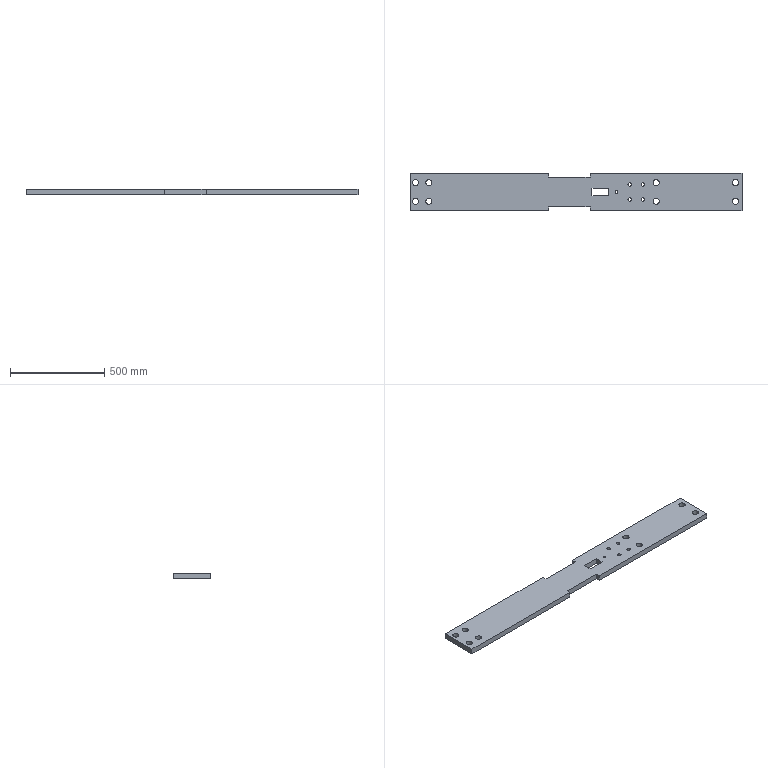Part | NX | features BREP 1, DATUM_CSYS 1, SKETCH 1 | 1 solid | 44 faces | box 1759 x 200 x 30 mm | volume 9929100 mm3 | cylinder 26 | plane 18 | commonest cylinder face diameters 18 x8 32 x8 33 x8 14 x2
STEP:
#1=CARTESIAN_POINT('',(-427.,0.,0.));
#2=VERTEX_POINT('',#1);
#3=CARTESIAN_POINT('',(-413.,0.,0.));
#4=VERTEX_POINT('',#3);
#5=CARTESIAN_POINT('',(-420.,0.,0.));
#6=DIRECTION('',(0.,0.,1.));
#7=DIRECTION('',(1.,0.,0.));
#8=AXIS2_PLACEMENT_3D('',#5,#6,#7);
#9=CIRCLE('',#8,7.);
#10=EDGE_CURVE('',#2,#4,#9,.T.);
#11=ORIENTED_EDGE('',*,*,#10,.F.);
#12=CARTESIAN_POINT('',(-427.,0.,30.));
#13=VERTEX_POINT('',#12);
#14=CARTESIAN_POINT('',(-427.,0.,0.));
#15=DIRECTION('',(0.,0.,1.));
#16=VECTOR('',#15,1000.);
#17=LINE('',#14,#16);
#18=EDGE_CURVE('',#2,#13,#17,.T.);
#19=ORIENTED_EDGE('',*,*,#18,.T.);
#20=CARTESIAN_POINT('',(-413.,0.,30.));
#21=VERTEX_POINT('',#20);
#22=CARTESIAN_POINT('',(-420.,0.,30.));
#23=DIRECTION('',(0.,0.,1.));
#24=DIRECTION('',(1.,0.,0.));
#25=AXIS2_PLACEMENT_3D('',#22,#23,#24);
#26=CIRCLE('',#25,7.);
#27=EDGE_CURVE('',#13,#21,#26,.T.);
#28=ORIENTED_EDGE('',*,*,#27,.T.);
#29=CARTESIAN_POINT('',(-413.,0.,0.));
#30=DIRECTION('',(0.,0.,1.));
#31=VECTOR('',#30,1000.);
#32=LINE('',#29,#31);
#33=EDGE_CURVE('',#4,#21,#32,.T.);
#34=ORIENTED_EDGE('',*,*,#33,.F.);
#35=EDGE_LOOP('',(#11,#19,#28,#34));
#36=FACE_BOUND('',#35,.T.);
#37=CARTESIAN_POINT('',(-420.,0.,0.));
#38=DIRECTION('',(0.,0.,1.));
#39=DIRECTION('',(-1.,0.,0.));
#40=AXIS2_PLACEMENT_3D('',#37,#38,#39);
#41=CYLINDRICAL_SURFACE('',#40,7.);
#42=ADVANCED_FACE('',(#36),#41,.F.);
#43=CARTESIAN_POINT('',(-1500.,50.,30.));
#44=VERTEX_POINT('',#43);
#45=CARTESIAN_POINT('',(-1468.,50.,30.));
#46=VERTEX_POINT('',#45);
#47=CARTESIAN_POINT('',(-1484.,50.,30.));
#48=DIRECTION('',(0.,0.,1.));
#49=DIRECTION('',(1.,0.,0.));
#50=AXIS2_PLACEMENT_3D('',#47,#48,#49);
#51=CIRCLE('',#50,16.);
#52=EDGE_CURVE('',#44,#46,#51,.T.);
#53=ORIENTED_EDGE('',*,*,#52,.T.);
#54=CARTESIAN_POINT('',(-1468.,50.,0.));
#55=VERTEX_POINT('',#54);
#56=CARTESIAN_POINT('',(-1468.,50.,30.));
#57=DIRECTION('',(0.,0.,-1.));
#58=VECTOR('',#57,1000.);
#59=LINE('',#56,#58);
#60=EDGE_CURVE('',#55,#46,#59,.F.);
#61=ORIENTED_EDGE('',*,*,#60,.F.);
#62=CARTESIAN_POINT('',(-1500.,50.,0.));
#63=VERTEX_POINT('',#62);
#64=CARTESIAN_POINT('',(-1484.,50.,0.));
#65=DIRECTION('',(0.,0.,1.));
#66=DIRECTION('',(1.,0.,0.));
#67=AXIS2_PLACEMENT_3D('',#64,#65,#66);
#68=CIRCLE('',#67,16.);
#69=EDGE_CURVE('',#63,#55,#68,.T.);
#70=ORIENTED_EDGE('',*,*,#69,.F.);
#71=CARTESIAN_POINT('',(-1500.,50.,30.));
#72=DIRECTION('',(0.,0.,-1.));
#73=VECTOR('',#72,1000.);
#74=LINE('',#71,#73);
#75=EDGE_CURVE('',#63,#44,#74,.F.);
#76=ORIENTED_EDGE('',*,*,#75,.T.);
#77=EDGE_LOOP('',(#53,#61,#70,#76));
#78=FACE_BOUND('',#77,.T.);
#79=CARTESIAN_POINT('',(-1484.,50.,30.));
#80=DIRECTION('',(0.,0.,-1.));
#81=DIRECTION('',(1.,0.,0.));
#82=AXIS2_PLACEMENT_3D('',#79,#80,#81);
#83=CYLINDRICAL_SURFACE('',#82,16.);
#84=ADVANCED_FACE('',(#78),#83,.F.);
#85=CARTESIAN_POINT('',(-1500.,-50.,30.));
#86=VERTEX_POINT('',#85);
#87=CARTESIAN_POINT('',(-1468.,-50.,30.));
#88=VERTEX_POINT('',#87);
#89=CARTESIAN_POINT('',(-1484.,-50.,30.));
#90=DIRECTION('',(0.,0.,1.));
#91=DIRECTION('',(1.,0.,0.));
#92=AXIS2_PLACEMENT_3D('',#89,#90,#91);
#93=CIRCLE('',#92,16.);
#94=EDGE_CURVE('',#86,#88,#93,.T.);
#95=ORIENTED_EDGE('',*,*,#94,.T.);
#96=CARTESIAN_POINT('',(-1468.,-50.,0.));
#97=VERTEX_POINT('',#96);
#98=CARTESIAN_POINT('',(-1468.,-50.,30.));
#99=DIRECTION('',(0.,0.,-1.));
#100=VECTOR('',#99,1000.);
#101=LINE('',#98,#100);
#102=EDGE_CURVE('',#97,#88,#101,.F.);
#103=ORIENTED_EDGE('',*,*,#102,.F.);
#104=CARTESIAN_POINT('',(-1500.,-50.,0.));
#105=VERTEX_POINT('',#104);
#106=CARTESIAN_POINT('',(-1484.,-50.,0.));
#107=DIRECTION('',(0.,0.,1.));
#108=DIRECTION('',(1.,0.,0.));
#109=AXIS2_PLACEMENT_3D('',#106,#107,#108);
#110=CIRCLE('',#109,16.);
#111=EDGE_CURVE('',#105,#97,#110,.T.);
#112=ORIENTED_EDGE('',*,*,#111,.F.);
#113=CARTESIAN_POINT('',(-1500.,-50.,30.));
#114=DIRECTION('',(0.,0.,-1.));
#115=VECTOR('',#114,1000.);
#116=LINE('',#113,#115);
#117=EDGE_CURVE('',#105,#86,#116,.F.);
#118=ORIENTED_EDGE('',*,*,#117,.T.);
#119=EDGE_LOOP('',(#95,#103,#112,#118));
#120=FACE_BOUND('',#119,.T.);
#121=CARTESIAN_POINT('',(-1484.,-50.,30.));
#122=DIRECTION('',(0.,0.,-1.));
#123=DIRECTION('',(1.,0.,0.));
#124=AXIS2_PLACEMENT_3D('',#121,#122,#123);
#125=CYLINDRICAL_SURFACE('',#124,16.);
#126=ADVANCED_FACE('',(#120),#125,.F.);
#127=CARTESIAN_POINT('',(-1430.,-50.,30.));
#128=VERTEX_POINT('',#127);
#129=CARTESIAN_POINT('',(-1398.,-50.,30.));
#130=VERTEX_POINT('',#129);
#131=CARTESIAN_POINT('',(-1414.,-50.,30.));
#132=DIRECTION('',(0.,0.,1.));
#133=DIRECTION('',(1.,0.,0.));
#134=AXIS2_PLACEMENT_3D('',#131,#132,#133);
#135=CIRCLE('',#134,16.);
#136=EDGE_CURVE('',#128,#130,#135,.T.);
#137=ORIENTED_EDGE('',*,*,#136,.T.);
#138=CARTESIAN_POINT('',(-1398.,-50.,0.));
#139=VERTEX_POINT('',#138);
#140=CARTESIAN_POINT('',(-1398.,-50.,30.));
#141=DIRECTION('',(0.,0.,-1.));
#142=VECTOR('',#141,1000.);
#143=LINE('',#140,#142);
#144=EDGE_CURVE('',#139,#130,#143,.F.);
#145=ORIENTED_EDGE('',*,*,#144,.F.);
#146=CARTESIAN_POINT('',(-1430.,-50.,0.));
#147=VERTEX_POINT('',#146);
#148=CARTESIAN_POINT('',(-1414.,-50.,0.));
#149=DIRECTION('',(0.,0.,1.));
#150=DIRECTION('',(1.,0.,0.));
#151=AXIS2_PLACEMENT_3D('',#148,#149,#150);
#152=CIRCLE('',#151,16.);
#153=EDGE_CURVE('',#147,#139,#152,.T.);
#154=ORIENTED_EDGE('',*,*,#153,.F.);
#155=CARTESIAN_POINT('',(-1430.,-50.,30.));
#156=DIRECTION('',(0.,0.,-1.));
#157=VECTOR('',#156,1000.);
#158=LINE('',#155,#157);
#159=EDGE_CURVE('',#147,#128,#158,.F.);
#160=ORIENTED_EDGE('',*,*,#159,.T.);
#161=EDGE_LOOP('',(#137,#145,#154,#160));
#162=FACE_BOUND('',#161,.T.);
#163=CARTESIAN_POINT('',(-1414.,-50.,30.));
#164=DIRECTION('',(0.,0.,-1.));
#165=DIRECTION('',(1.,0.,0.));
#166=AXIS2_PLACEMENT_3D('',#163,#164,#165);
#167=CYLINDRICAL_SURFACE('',#166,16.);
#168=ADVANCED_FACE('',(#162),#167,.F.);
#169=CARTESIAN_POINT('',(-1430.,50.,30.));
#170=VERTEX_POINT('',#169);
#171=CARTESIAN_POINT('',(-1398.,50.,30.));
#172=VERTEX_POINT('',#171);
#173=CARTESIAN_POINT('',(-1414.,50.,30.));
#174=DIRECTION('',(0.,0.,1.));
#175=DIRECTION('',(1.,0.,0.));
#176=AXIS2_PLACEMENT_3D('',#173,#174,#175);
#177=CIRCLE('',#176,16.);
#178=EDGE_CURVE('',#170,#172,#177,.T.);
#179=ORIENTED_EDGE('',*,*,#178,.T.);
#180=CARTESIAN_POINT('',(-1398.,50.,0.));
#181=VERTEX_POINT('',#180);
#182=CARTESIAN_POINT('',(-1398.,50.,30.));
#183=DIRECTION('',(0.,0.,-1.));
#184=VECTOR('',#183,1000.);
#185=LINE('',#182,#184);
#186=EDGE_CURVE('',#181,#172,#185,.F.);
#187=ORIENTED_EDGE('',*,*,#186,.F.);
#188=CARTESIAN_POINT('',(-1430.,50.,0.));
#189=VERTEX_POINT('',#188);
#190=CARTESIAN_POINT('',(-1414.,50.,0.));
#191=DIRECTION('',(0.,0.,1.));
#192=DIRECTION('',(1.,0.,0.));
#193=AXIS2_PLACEMENT_3D('',#190,#191,#192);
#194=CIRCLE('',#193,16.);
#195=EDGE_CURVE('',#189,#181,#194,.T.);
#196=ORIENTED_EDGE('',*,*,#195,.F.);
#197=CARTESIAN_POINT('',(-1430.,50.,30.));
#198=DIRECTION('',(0.,0.,-1.));
#199=VECTOR('',#198,1000.);
#200=LINE('',#197,#199);
#201=EDGE_CURVE('',#189,#170,#200,.F.);
#202=ORIENTED_EDGE('',*,*,#201,.T.);
#203=EDGE_LOOP('',(#179,#187,#196,#202));
#204=FACE_BOUND('',#203,.T.);
#205=CARTESIAN_POINT('',(-1414.,50.,30.));
#206=DIRECTION('',(0.,0.,-1.));
#207=DIRECTION('',(1.,0.,0.));
#208=AXIS2_PLACEMENT_3D('',#205,#206,#207);
#209=CYLINDRICAL_SURFACE('',#208,16.);
#210=ADVANCED_FACE('',(#204),#209,.F.);
#211=CARTESIAN_POINT('',(-359.,-40.,30.));
#212=VERTEX_POINT('',#211);
#213=CARTESIAN_POINT('',(-341.,-40.,30.));
#214=VERTEX_POINT('',#213);
#215=CARTESIAN_POINT('',(-350.,-40.,30.));
#216=DIRECTION('',(0.,0.,1.));
#217=DIRECTION('',(1.,0.,0.));
#218=AXIS2_PLACEMENT_3D('',#215,#216,#217);
#219=CIRCLE('',#218,9.);
#220=EDGE_CURVE('',#212,#214,#219,.T.);
#221=ORIENTED_EDGE('',*,*,#220,.T.);
#222=CARTESIAN_POINT('',(-341.,-40.,0.));
#223=VERTEX_POINT('',#222);
#224=CARTESIAN_POINT('',(-341.,-40.,30.));
#225=DIRECTION('',(0.,0.,-1.));
#226=VECTOR('',#225,1000.);
#227=LINE('',#224,#226);
#228=EDGE_CURVE('',#223,#214,#227,.F.);
#229=ORIENTED_EDGE('',*,*,#228,.F.);
#230=CARTESIAN_POINT('',(-359.,-40.,0.));
#231=VERTEX_POINT('',#230);
#232=CARTESIAN_POINT('',(-350.,-40.,0.));
#233=DIRECTION('',(0.,0.,1.));
#234=DIRECTION('',(1.,0.,0.));
#235=AXIS2_PLACEMENT_3D('',#232,#233,#234);
#236=CIRCLE('',#235,9.);
#237=EDGE_CURVE('',#231,#223,#236,.T.);
#238=ORIENTED_EDGE('',*,*,#237,.F.);
#239=CARTESIAN_POINT('',(-359.,-40.,30.));
#240=DIRECTION('',(0.,0.,-1.));
#241=VECTOR('',#240,1000.);
#242=LINE('',#239,#241);
#243=EDGE_CURVE('',#231,#212,#242,.F.);
#244=ORIENTED_EDGE('',*,*,#243,.T.);
#245=EDGE_LOOP('',(#221,#229,#238,#244));
#246=FACE_BOUND('',#245,.T.);
#247=CARTESIAN_POINT('',(-350.,-40.,30.));
#248=DIRECTION('',(0.,0.,-1.));
#249=DIRECTION('',(1.,0.,0.));
#250=AXIS2_PLACEMENT_3D('',#247,#248,#249);
#251=CYLINDRICAL_SURFACE('',#250,9.);
#252=ADVANCED_FACE('',(#246),#251,.F.);
#253=CARTESIAN_POINT('',(-289.,-40.,30.));
#254=VERTEX_POINT('',#253);
#255=CARTESIAN_POINT('',(-271.,-40.,30.));
#256=VERTEX_POINT('',#255);
#257=CARTESIAN_POINT('',(-280.,-40.,30.));
#258=DIRECTION('',(0.,0.,1.));
#259=DIRECTION('',(1.,0.,0.));
#260=AXIS2_PLACEMENT_3D('',#257,#258,#259);
#261=CIRCLE('',#260,9.);
#262=EDGE_CURVE('',#254,#256,#261,.T.);
#263=ORIENTED_EDGE('',*,*,#262,.T.);
#264=CARTESIAN_POINT('',(-271.,-40.,0.));
#265=VERTEX_POINT('',#264);
#266=CARTESIAN_POINT('',(-271.,-40.,30.));
#267=DIRECTION('',(0.,0.,-1.));
#268=VECTOR('',#267,1000.);
#269=LINE('',#266,#268);
#270=EDGE_CURVE('',#265,#256,#269,.F.);
#271=ORIENTED_EDGE('',*,*,#270,.F.);
#272=CARTESIAN_POINT('',(-289.,-40.,0.));
#273=VERTEX_POINT('',#272);
#274=CARTESIAN_POINT('',(-280.,-40.,0.));
#275=DIRECTION('',(0.,0.,1.));
#276=DIRECTION('',(1.,0.,0.));
#277=AXIS2_PLACEMENT_3D('',#274,#275,#276);
#278=CIRCLE('',#277,9.);
#279=EDGE_CURVE('',#273,#265,#278,.T.);
#280=ORIENTED_EDGE('',*,*,#279,.F.);
#281=CARTESIAN_POINT('',(-289.,-40.,30.));
#282=DIRECTION('',(0.,0.,-1.));
#283=VECTOR('',#282,1000.);
#284=LINE('',#281,#283);
#285=EDGE_CURVE('',#273,#254,#284,.F.);
#286=ORIENTED_EDGE('',*,*,#285,.T.);
#287=EDGE_LOOP('',(#263,#271,#280,#286));
#288=FACE_BOUND('',#287,.T.);
#289=CARTESIAN_POINT('',(-280.,-40.,30.));
#290=DIRECTION('',(0.,0.,-1.));
#291=DIRECTION('',(1.,0.,0.));
#292=AXIS2_PLACEMENT_3D('',#289,#290,#291);
#293=CYLINDRICAL_SURFACE('',#292,9.);
#294=ADVANCED_FACE('',(#288),#293,.F.);
#295=CARTESIAN_POINT('',(-289.,40.,30.));
#296=VERTEX_POINT('',#295);
#297=CARTESIAN_POINT('',(-271.,40.,30.));
#298=VERTEX_POINT('',#297);
#299=CARTESIAN_POINT('',(-280.,40.,30.));
#300=DIRECTION('',(0.,0.,1.));
#301=DIRECTION('',(1.,0.,0.));
#302=AXIS2_PLACEMENT_3D('',#299,#300,#301);
#303=CIRCLE('',#302,9.);
#304=EDGE_CURVE('',#296,#298,#303,.T.);
#305=ORIENTED_EDGE('',*,*,#304,.T.);
#306=CARTESIAN_POINT('',(-271.,40.,0.));
#307=VERTEX_POINT('',#306);
#308=CARTESIAN_POINT('',(-271.,40.,30.));
#309=DIRECTION('',(0.,0.,-1.));
#310=VECTOR('',#309,1000.);
#311=LINE('',#308,#310);
#312=EDGE_CURVE('',#307,#298,#311,.F.);
#313=ORIENTED_EDGE('',*,*,#312,.F.);
#314=CARTESIAN_POINT('',(-289.,40.,0.));
#315=VERTEX_POINT('',#314);
#316=CARTESIAN_POINT('',(-280.,40.,0.));
#317=DIRECTION('',(0.,0.,1.));
#318=DIRECTION('',(1.,0.,0.));
#319=AXIS2_PLACEMENT_3D('',#316,#317,#318);
#320=CIRCLE('',#319,9.);
#321=EDGE_CURVE('',#315,#307,#320,.T.);
#322=ORIENTED_EDGE('',*,*,#321,.F.);
#323=CARTESIAN_POINT('',(-289.,40.,30.));
#324=DIRECTION('',(0.,0.,-1.));
#325=VECTOR('',#324,1000.);
#326=LINE('',#323,#325);
#327=EDGE_CURVE('',#315,#296,#326,.F.);
#328=ORIENTED_EDGE('',*,*,#327,.T.);
#329=EDGE_LOOP('',(#305,#313,#322,#328));
#330=FACE_BOUND('',#329,.T.);
#331=CARTESIAN_POINT('',(-280.,40.,30.));
#332=DIRECTION('',(0.,0.,-1.));
#333=DIRECTION('',(1.,0.,0.));
#334=AXIS2_PLACEMENT_3D('',#331,#332,#333);
#335=CYLINDRICAL_SURFACE('',#334,9.);
#336=ADVANCED_FACE('',(#330),#335,.F.);
#337=CARTESIAN_POINT('',(-359.,40.,30.));
#338=VERTEX_POINT('',#337);
#339=CARTESIAN_POINT('',(-341.,40.,30.));
#340=VERTEX_POINT('',#339);
#341=CARTESIAN_POINT('',(-350.,40.,30.));
#342=DIRECTION('',(0.,0.,1.));
#343=DIRECTION('',(1.,0.,0.));
#344=AXIS2_PLACEMENT_3D('',#341,#342,#343);
#345=CIRCLE('',#344,9.);
#346=EDGE_CURVE('',#338,#340,#345,.T.);
#347=ORIENTED_EDGE('',*,*,#346,.T.);
#348=CARTESIAN_POINT('',(-341.,40.,0.));
#349=VERTEX_POINT('',#348);
#350=CARTESIAN_POINT('',(-341.,40.,30.));
#351=DIRECTION('',(0.,0.,-1.));
#352=VECTOR('',#351,1000.);
#353=LINE('',#350,#352);
#354=EDGE_CURVE('',#349,#340,#353,.F.);
#355=ORIENTED_EDGE('',*,*,#354,.F.);
#356=CARTESIAN_POINT('',(-359.,40.,0.));
#357=VERTEX_POINT('',#356);
#358=CARTESIAN_POINT('',(-350.,40.,0.));
#359=DIRECTION('',(0.,0.,1.));
#360=DIRECTION('',(1.,0.,0.));
#361=AXIS2_PLACEMENT_3D('',#358,#359,#360);
#362=CIRCLE('',#361,9.);
#363=EDGE_CURVE('',#357,#349,#362,.T.);
#364=ORIENTED_EDGE('',*,*,#363,.F.);
#365=CARTESIAN_POINT('',(-359.,40.,30.));
#366=DIRECTION('',(0.,0.,-1.));
#367=VECTOR('',#366,1000.);
#368=LINE('',#365,#367);
#369=EDGE_CURVE('',#357,#338,#368,.F.);
#370=ORIENTED_EDGE('',*,*,#369,.T.);
#371=EDGE_LOOP('',(#347,#355,#364,#370));
#372=FACE_BOUND('',#371,.T.);
#373=CARTESIAN_POINT('',(-350.,40.,30.));
#374=DIRECTION('',(0.,0.,-1.));
#375=DIRECTION('',(1.,0.,0.));
#376=AXIS2_PLACEMENT_3D('',#373,#374,#375);
#377=CYLINDRICAL_SURFACE('',#376,9.);
#378=ADVANCED_FACE('',(#372),#377,.F.);
#379=CARTESIAN_POINT('',(-226.5,50.,30.));
#380=VERTEX_POINT('',#379);
#381=CARTESIAN_POINT('',(-193.5,50.,30.));
#382=VERTEX_POINT('',#381);
#383=CARTESIAN_POINT('',(-210.,50.,30.));
#384=DIRECTION('',(0.,0.,1.));
#385=DIRECTION('',(1.,0.,0.));
#386=AXIS2_PLACEMENT_3D('',#383,#384,#385);
#387=CIRCLE('',#386,16.5);
#388=EDGE_CURVE('',#380,#382,#387,.T.);
#389=ORIENTED_EDGE('',*,*,#388,.T.);
#390=CARTESIAN_POINT('',(-193.5,50.,0.));
#391=VERTEX_POINT('',#390);
#392=CARTESIAN_POINT('',(-193.5,50.,30.));
#393=DIRECTION('',(0.,0.,-1.));
#394=VECTOR('',#393,1000.);
#395=LINE('',#392,#394);
#396=EDGE_CURVE('',#391,#382,#395,.F.);
#397=ORIENTED_EDGE('',*,*,#396,.F.);
#398=CARTESIAN_POINT('',(-226.5,50.,0.));
#399=VERTEX_POINT('',#398);
#400=CARTESIAN_POINT('',(-210.,50.,0.));
#401=DIRECTION('',(0.,0.,1.));
#402=DIRECTION('',(1.,0.,0.));
#403=AXIS2_PLACEMENT_3D('',#400,#401,#402);
#404=CIRCLE('',#403,16.5);
#405=EDGE_CURVE('',#399,#391,#404,.T.);
#406=ORIENTED_EDGE('',*,*,#405,.F.);
#407=CARTESIAN_POINT('',(-226.5,50.,30.));
#408=DIRECTION('',(0.,0.,-1.));
#409=VECTOR('',#408,1000.);
#410=LINE('',#407,#409);
#411=EDGE_CURVE('',#399,#380,#410,.F.);
#412=ORIENTED_EDGE('',*,*,#411,.T.);
#413=EDGE_LOOP('',(#389,#397,#406,#412));
#414=FACE_BOUND('',#413,.T.);
#415=CARTESIAN_POINT('',(-210.,50.,30.));
#416=DIRECTION('',(0.,0.,-1.));
#417=DIRECTION('',(1.,0.,0.));
#418=AXIS2_PLACEMENT_3D('',#415,#416,#417);
#419=CYLINDRICAL_SURFACE('',#418,16.5);
#420=ADVANCED_FACE('',(#414),#419,.F.);
#421=CARTESIAN_POINT('',(-226.5,-50.,30.));
#422=VERTEX_POINT('',#421);
#423=CARTESIAN_POINT('',(-193.5,-50.,30.));
#424=VERTEX_POINT('',#423);
#425=CARTESIAN_POINT('',(-210.,-50.,30.));
#426=DIRECTION('',(0.,0.,1.));
#427=DIRECTION('',(1.,0.,0.));
#428=AXIS2_PLACEMENT_3D('',#425,#426,#427);
#429=CIRCLE('',#428,16.5);
#430=EDGE_CURVE('',#422,#424,#429,.T.);
#431=ORIENTED_EDGE('',*,*,#430,.T.);
#432=CARTESIAN_POINT('',(-193.5,-50.,0.));
#433=VERTEX_POINT('',#432);
#434=CARTESIAN_POINT('',(-193.5,-50.,30.));
#435=DIRECTION('',(0.,0.,-1.));
#436=VECTOR('',#435,1000.);
#437=LINE('',#434,#436);
#438=EDGE_CURVE('',#433,#424,#437,.F.);
#439=ORIENTED_EDGE('',*,*,#438,.F.);
#440=CARTESIAN_POINT('',(-226.5,-50.,0.));
#441=VERTEX_POINT('',#440);
#442=CARTESIAN_POINT('',(-210.,-50.,0.));
#443=DIRECTION('',(0.,0.,1.));
#444=DIRECTION('',(1.,0.,0.));
#445=AXIS2_PLACEMENT_3D('',#442,#443,#444);
#446=CIRCLE('',#445,16.5);
#447=EDGE_CURVE('',#441,#433,#446,.T.);
#448=ORIENTED_EDGE('',*,*,#447,.F.);
#449=CARTESIAN_POINT('',(-226.5,-50.,30.));
#450=DIRECTION('',(0.,0.,-1.));
#451=VECTOR('',#450,1000.);
#452=LINE('',#449,#451);
#453=EDGE_CURVE('',#441,#422,#452,.F.);
#454=ORIENTED_EDGE('',*,*,#453,.T.);
#455=EDGE_LOOP('',(#431,#439,#448,#454));
#456=FACE_BOUND('',#455,.T.);
#457=CARTESIAN_POINT('',(-210.,-50.,30.));
#458=DIRECTION('',(0.,0.,-1.));
#459=DIRECTION('',(1.,0.,0.));
#460=AXIS2_PLACEMENT_3D('',#457,#458,#459);
#461=CYLINDRICAL_SURFACE('',#460,16.5);
#462=ADVANCED_FACE('',(#456),#461,.F.);
#463=CARTESIAN_POINT('',(193.5,-50.,30.));
#464=VERTEX_POINT('',#463);
#465=CARTESIAN_POINT('',(226.5,-50.,30.));
#466=VERTEX_POINT('',#465);
#467=CARTESIAN_POINT('',(210.,-50.,30.));
#468=DIRECTION('',(0.,0.,1.));
#469=DIRECTION('',(1.,0.,0.));
#470=AXIS2_PLACEMENT_3D('',#467,#468,#469);
#471=CIRCLE('',#470,16.5);
#472=EDGE_CURVE('',#464,#466,#471,.T.);
#473=ORIENTED_EDGE('',*,*,#472,.T.);
#474=CARTESIAN_POINT('',(226.5,-50.,0.));
#475=VERTEX_POINT('',#474);
#476=CARTESIAN_POINT('',(226.5,-50.,30.));
#477=DIRECTION('',(0.,0.,-1.));
#478=VECTOR('',#477,1000.);
#479=LINE('',#476,#478);
#480=EDGE_CURVE('',#475,#466,#479,.F.);
#481=ORIENTED_EDGE('',*,*,#480,.F.);
#482=CARTESIAN_POINT('',(193.5,-50.,0.));
#483=VERTEX_POINT('',#482);
#484=CARTESIAN_POINT('',(210.,-50.,0.));
#485=DIRECTION('',(0.,0.,1.));
#486=DIRECTION('',(1.,0.,0.));
#487=AXIS2_PLACEMENT_3D('',#484,#485,#486);
#488=CIRCLE('',#487,16.5);
#489=EDGE_CURVE('',#483,#475,#488,.T.);
#490=ORIENTED_EDGE('',*,*,#489,.F.);
#491=CARTESIAN_POINT('',(193.5,-50.,30.));
#492=DIRECTION('',(0.,0.,-1.));
#493=VECTOR('',#492,1000.);
#494=LINE('',#491,#493);
#495=EDGE_CURVE('',#483,#464,#494,.F.);
#496=ORIENTED_EDGE('',*,*,#495,.T.);
#497=EDGE_LOOP('',(#473,#481,#490,#496));
#498=FACE_BOUND('',#497,.T.);
#499=CARTESIAN_POINT('',(210.,-50.,30.));
#500=DIRECTION('',(0.,0.,-1.));
#501=DIRECTION('',(1.,0.,0.));
#502=AXIS2_PLACEMENT_3D('',#499,#500,#501);
#503=CYLINDRICAL_SURFACE('',#502,16.5);
#504=ADVANCED_FACE('',(#498),#503,.F.);
#505=CARTESIAN_POINT('',(193.5,50.,30.));
#506=VERTEX_POINT('',#505);
#507=CARTESIAN_POINT('',(226.5,50.,30.));
#508=VERTEX_POINT('',#507);
#509=CARTESIAN_POINT('',(210.,50.,30.));
#510=DIRECTION('',(0.,0.,1.));
#511=DIRECTION('',(1.,0.,0.));
#512=AXIS2_PLACEMENT_3D('',#509,#510,#511);
#513=CIRCLE('',#512,16.5);
#514=EDGE_CURVE('',#506,#508,#513,.T.);
#515=ORIENTED_EDGE('',*,*,#514,.T.);
#516=CARTESIAN_POINT('',(226.5,50.,0.));
#517=VERTEX_POINT('',#516);
#518=CARTESIAN_POINT('',(226.5,50.,30.));
#519=DIRECTION('',(0.,0.,-1.));
#520=VECTOR('',#519,1000.);
#521=LINE('',#518,#520);
#522=EDGE_CURVE('',#517,#508,#521,.F.);
#523=ORIENTED_EDGE('',*,*,#522,.F.);
#524=CARTESIAN_POINT('',(193.5,50.,0.));
#525=VERTEX_POINT('',#524);
#526=CARTESIAN_POINT('',(210.,50.,0.));
#527=DIRECTION('',(0.,0.,1.));
#528=DIRECTION('',(1.,0.,0.));
#529=AXIS2_PLACEMENT_3D('',#526,#527,#528);
#530=CIRCLE('',#529,16.5);
#531=EDGE_CURVE('',#525,#517,#530,.T.);
#532=ORIENTED_EDGE('',*,*,#531,.F.);
#533=CARTESIAN_POINT('',(193.5,50.,30.));
#534=DIRECTION('',(0.,0.,-1.));
#535=VECTOR('',#534,1000.);
#536=LINE('',#533,#535);
#537=EDGE_CURVE('',#525,#506,#536,.F.);
#538=ORIENTED_EDGE('',*,*,#537,.T.);
#539=EDGE_LOOP('',(#515,#523,#532,#538));
#540=FACE_BOUND('',#539,.T.);
#541=CARTESIAN_POINT('',(210.,50.,30.));
#542=DIRECTION('',(0.,0.,-1.));
#543=DIRECTION('',(1.,0.,0.));
#544=AXIS2_PLACEMENT_3D('',#541,#542,#543);
#545=CYLINDRICAL_SURFACE('',#544,16.5);
#546=ADVANCED_FACE('',(#540),#545,.F.);
#547=CARTESIAN_POINT('',(-420.,0.,30.));
#548=DIRECTION('',(0.,0.,1.));
#549=DIRECTION('',(1.,0.,0.));
#550=AXIS2_PLACEMENT_3D('',#547,#548,#549);
#551=CIRCLE('',#550,7.);
#552=EDGE_CURVE('',#21,#13,#551,.T.);
#553=ORIENTED_EDGE('',*,*,#552,.F.);
#554=ORIENTED_EDGE('',*,*,#27,.F.);
#555=EDGE_LOOP('',(#553,#554));
#556=FACE_BOUND('',#555,.T.);
#557=CARTESIAN_POINT('',(-550.,-21.,30.));
#558=VERTEX_POINT('',#557);
#559=CARTESIAN_POINT('',(-460.,-21.,30.));
#560=VERTEX_POINT('',#559);
#561=CARTESIAN_POINT('',(-550.,-21.,30.));
#562=DIRECTION('',(1.,0.,0.));
#563=VECTOR('',#562,1000.);
#564=LINE('',#561,#563);
#565=EDGE_CURVE('',#558,#560,#564,.T.);
#566=ORIENTED_EDGE('',*,*,#565,.F.);
#567=CARTESIAN_POINT('',(-550.,21.,30.));
#568=VERTEX_POINT('',#567);
#569=CARTESIAN_POINT('',(-550.,-21.,30.));
#570=DIRECTION('',(0.,-1.,0.));
#571=VECTOR('',#570,1000.);
#572=LINE('',#569,#571);
#573=EDGE_CURVE('',#568,#558,#572,.T.);
#574=ORIENTED_EDGE('',*,*,#573,.F.);
#575=CARTESIAN_POINT('',(-460.,21.,30.));
#576=VERTEX_POINT('',#575);
#577=CARTESIAN_POINT('',(-550.,21.,30.));
#578=DIRECTION('',(-1.,0.,0.));
#579=VECTOR('',#578,1000.);
#580=LINE('',#577,#579);
#581=EDGE_CURVE('',#576,#568,#580,.T.);
#582=ORIENTED_EDGE('',*,*,#581,.F.);
#583=CARTESIAN_POINT('',(-460.,-21.,30.));
#584=DIRECTION('',(0.,1.,0.));
#585=VECTOR('',#584,1000.);
#586=LINE('',#583,#585);
#587=EDGE_CURVE('',#560,#576,#586,.T.);
#588=ORIENTED_EDGE('',*,*,#587,.F.);
#589=EDGE_LOOP('',(#566,#574,#582,#588));
#590=FACE_BOUND('',#589,.T.);
#591=ORIENTED_EDGE('',*,*,#94,.F.);
#592=CARTESIAN_POINT('',(-1484.,-50.,30.));
#593=DIRECTION('',(0.,0.,1.));
#594=DIRECTION('',(1.,0.,0.));
#595=AXIS2_PLACEMENT_3D('',#592,#593,#594);
#596=CIRCLE('',#595,16.);
#597=EDGE_CURVE('',#88,#86,#596,.T.);
#598=ORIENTED_EDGE('',*,*,#597,.F.);
#599=EDGE_LOOP('',(#591,#598));
#600=FACE_BOUND('',#599,.T.);
#601=ORIENTED_EDGE('',*,*,#178,.F.);
#602=CARTESIAN_POINT('',(-1414.,50.,30.));
#603=DIRECTION('',(0.,0.,1.));
#604=DIRECTION('',(1.,0.,0.));
#605=AXIS2_PLACEMENT_3D('',#602,#603,#604);
#606=CIRCLE('',#605,16.);
#607=EDGE_CURVE('',#172,#170,#606,.T.);
#608=ORIENTED_EDGE('',*,*,#607,.F.);
#609=EDGE_LOOP('',(#601,#608));
#610=FACE_BOUND('',#609,.T.);
#611=ORIENTED_EDGE('',*,*,#262,.F.);
#612=CARTESIAN_POINT('',(-280.,-40.,30.));
#613=DIRECTION('',(0.,0.,1.));
#614=DIRECTION('',(1.,0.,0.));
#615=AXIS2_PLACEMENT_3D('',#612,#613,#614);
#616=CIRCLE('',#615,9.);
#617=EDGE_CURVE('',#256,#254,#616,.T.);
#618=ORIENTED_EDGE('',*,*,#617,.F.);
#619=EDGE_LOOP('',(#611,#618));
#620=FACE_BOUND('',#619,.T.);
#621=ORIENTED_EDGE('',*,*,#346,.F.);
#622=CARTESIAN_POINT('',(-350.,40.,30.));
#623=DIRECTION('',(0.,0.,1.));
#624=DIRECTION('',(1.,0.,0.));
#625=AXIS2_PLACEMENT_3D('',#622,#623,#624);
#626=CIRCLE('',#625,9.);
#627=EDGE_CURVE('',#340,#338,#626,.T.);
#628=ORIENTED_EDGE('',*,*,#627,.F.);
#629=EDGE_LOOP('',(#621,#628));
#630=FACE_BOUND('',#629,.T.);
#631=ORIENTED_EDGE('',*,*,#430,.F.);
#632=CARTESIAN_POINT('',(-210.,-50.,30.));
#633=DIRECTION('',(0.,0.,1.));
#634=DIRECTION('',(1.,0.,0.));
#635=AXIS2_PLACEMENT_3D('',#632,#633,#634);
#636=CIRCLE('',#635,16.5);
#637=EDGE_CURVE('',#424,#422,#636,.T.);
#638=ORIENTED_EDGE('',*,*,#637,.F.);
#639=EDGE_LOOP('',(#631,#638));
#640=FACE_BOUND('',#639,.T.);
#641=ORIENTED_EDGE('',*,*,#514,.F.);
#642=CARTESIAN_POINT('',(210.,50.,30.));
#643=DIRECTION('',(0.,0.,1.));
#644=DIRECTION('',(1.,0.,0.));
#645=AXIS2_PLACEMENT_3D('',#642,#643,#644);
#646=CIRCLE('',#645,16.5);
#647=EDGE_CURVE('',#508,#506,#646,.T.);
#648=ORIENTED_EDGE('',*,*,#647,.F.);
#649=EDGE_LOOP('',(#641,#648));
#650=FACE_BOUND('',#649,.T.);
#651=CARTESIAN_POINT('',(245.,-100.,30.));
#652=VERTEX_POINT('',#651);
#653=CARTESIAN_POINT('',(245.,100.,30.));
#654=VERTEX_POINT('',#653);
#655=CARTESIAN_POINT('',(245.,100.,30.));
#656=DIRECTION('',(0.,1.,0.));
#657=VECTOR('',#656,1000.);
#658=LINE('',#655,#657);
#659=EDGE_CURVE('',#652,#654,#658,.T.);
#660=ORIENTED_EDGE('',*,*,#659,.T.);
#661=CARTESIAN_POINT('',(-560.,100.,30.));
#662=VERTEX_POINT('',#661);
#663=CARTESIAN_POINT('',(245.,100.,30.));
#664=DIRECTION('',(-1.,0.,0.));
#665=VECTOR('',#664,1000.);
#666=LINE('',#663,#665);
#667=EDGE_CURVE('',#654,#662,#666,.T.);
#668=ORIENTED_EDGE('',*,*,#667,.T.);
#669=CARTESIAN_POINT('',(-560.,79.,30.));
#670=VERTEX_POINT('',#669);
#671=CARTESIAN_POINT('',(-560.,100.,30.));
#672=DIRECTION('',(0.,-1.,0.));
#673=VECTOR('',#672,1000.);
#674=LINE('',#671,#673);
#675=EDGE_CURVE('',#662,#670,#674,.T.);
#676=ORIENTED_EDGE('',*,*,#675,.T.);
#677=CARTESIAN_POINT('',(-780.,79.,30.));
#678=VERTEX_POINT('',#677);
#679=CARTESIAN_POINT('',(-780.,79.,30.));
#680=DIRECTION('',(-1.,0.,0.));
#681=VECTOR('',#680,1000.);
#682=LINE('',#679,#681);
#683=EDGE_CURVE('',#670,#678,#682,.T.);
#684=ORIENTED_EDGE('',*,*,#683,.T.);
#685=CARTESIAN_POINT('',(-780.,100.,30.));
#686=VERTEX_POINT('',#685);
#687=CARTESIAN_POINT('',(-780.,100.,30.));
#688=DIRECTION('',(0.,1.,0.));
#689=VECTOR('',#688,1000.);
#690=LINE('',#687,#689);
#691=EDGE_CURVE('',#678,#686,#690,.T.);
#692=ORIENTED_EDGE('',*,*,#691,.T.);
#693=CARTESIAN_POINT('',(-1514.,100.,30.));
#694=VERTEX_POINT('',#693);
#695=CARTESIAN_POINT('',(-780.,100.,30.));
#696=DIRECTION('',(-1.,0.,0.));
#697=VECTOR('',#696,1000.);
#698=LINE('',#695,#697);
#699=EDGE_CURVE('',#686,#694,#698,.T.);
#700=ORIENTED_EDGE('',*,*,#699,.T.);
#701=CARTESIAN_POINT('',(-1514.,-100.,30.));
#702=VERTEX_POINT('',#701);
#703=CARTESIAN_POINT('',(-1514.,100.,30.));
#704=DIRECTION('',(0.,-1.,0.));
#705=VECTOR('',#704,1000.);
#706=LINE('',#703,#705);
#707=EDGE_CURVE('',#694,#702,#706,.T.);
#708=ORIENTED_EDGE('',*,*,#707,.T.);
#709=CARTESIAN_POINT('',(-780.,-100.,30.));
#710=VERTEX_POINT('',#709);
#711=CARTESIAN_POINT('',(-780.,-100.,30.));
#712=DIRECTION('',(1.,0.,0.));
#713=VECTOR('',#712,1000.);
#714=LINE('',#711,#713);
#715=EDGE_CURVE('',#702,#710,#714,.T.);
#716=ORIENTED_EDGE('',*,*,#715,.T.);
#717=CARTESIAN_POINT('',(-780.,-79.,30.));
#718=VERTEX_POINT('',#717);
#719=CARTESIAN_POINT('',(-780.,-79.,30.));
#720=DIRECTION('',(0.,1.,0.));
#721=VECTOR('',#720,1000.);
#722=LINE('',#719,#721);
#723=EDGE_CURVE('',#710,#718,#722,.T.);
#724=ORIENTED_EDGE('',*,*,#723,.T.);
#725=CARTESIAN_POINT('',(-560.,-79.,30.));
#726=VERTEX_POINT('',#725);
#727=CARTESIAN_POINT('',(-780.,-79.,30.));
#728=DIRECTION('',(1.,0.,0.));
#729=VECTOR('',#728,1000.);
#730=LINE('',#727,#729);
#731=EDGE_CURVE('',#718,#726,#730,.T.);
#732=ORIENTED_EDGE('',*,*,#731,.T.);
#733=CARTESIAN_POINT('',(-560.,-100.,30.));
#734=VERTEX_POINT('',#733);
#735=CARTESIAN_POINT('',(-560.,-79.,30.));
#736=DIRECTION('',(0.,-1.,0.));
#737=VECTOR('',#736,1000.);
#738=LINE('',#735,#737);
#739=EDGE_CURVE('',#726,#734,#738,.T.);
#740=ORIENTED_EDGE('',*,*,#739,.T.);
#741=CARTESIAN_POINT('',(245.,-100.,30.));
#742=DIRECTION('',(1.,0.,0.));
#743=VECTOR('',#742,1000.);
#744=LINE('',#741,#743);
#745=EDGE_CURVE('',#734,#652,#744,.T.);
#746=ORIENTED_EDGE('',*,*,#745,.T.);
#747=EDGE_LOOP('',(#660,#668,#676,#684,#692,#700,#708,#716,#724,#732,#740,#746));
#748=FACE_BOUND('',#747,.T.);
#749=ORIENTED_EDGE('',*,*,#472,.F.);
#750=CARTESIAN_POINT('',(210.,-50.,30.));
#751=DIRECTION('',(0.,0.,1.));
#752=DIRECTION('',(1.,0.,0.));
#753=AXIS2_PLACEMENT_3D('',#750,#751,#752);
#754=CIRCLE('',#753,16.5);
#755=EDGE_CURVE('',#466,#464,#754,.T.);
#756=ORIENTED_EDGE('',*,*,#755,.F.);
#757=EDGE_LOOP('',(#749,#756));
#758=FACE_BOUND('',#757,.T.);
#759=ORIENTED_EDGE('',*,*,#388,.F.);
#760=CARTESIAN_POINT('',(-210.,50.,30.));
#761=DIRECTION('',(0.,0.,1.));
#762=DIRECTION('',(1.,0.,0.));
#763=AXIS2_PLACEMENT_3D('',#760,#761,#762);
#764=CIRCLE('',#763,16.5);
#765=EDGE_CURVE('',#382,#380,#764,.T.);
#766=ORIENTED_EDGE('',*,*,#765,.F.);
#767=EDGE_LOOP('',(#759,#766));
#768=FACE_BOUND('',#767,.T.);
#769=ORIENTED_EDGE('',*,*,#304,.F.);
#770=CARTESIAN_POINT('',(-280.,40.,30.));
#771=DIRECTION('',(0.,0.,1.));
#772=DIRECTION('',(1.,0.,0.));
#773=AXIS2_PLACEMENT_3D('',#770,#771,#772);
#774=CIRCLE('',#773,9.);
#775=EDGE_CURVE('',#298,#296,#774,.T.);
#776=ORIENTED_EDGE('',*,*,#775,.F.);
#777=EDGE_LOOP('',(#769,#776));
#778=FACE_BOUND('',#777,.T.);
#779=ORIENTED_EDGE('',*,*,#220,.F.);
#780=CARTESIAN_POINT('',(-350.,-40.,30.));
#781=DIRECTION('',(0.,0.,1.));
#782=DIRECTION('',(1.,0.,0.));
#783=AXIS2_PLACEMENT_3D('',#780,#781,#782);
#784=CIRCLE('',#783,9.);
#785=EDGE_CURVE('',#214,#212,#784,.T.);
#786=ORIENTED_EDGE('',*,*,#785,.F.);
#787=EDGE_LOOP('',(#779,#786));
#788=FACE_BOUND('',#787,.T.);
#789=ORIENTED_EDGE('',*,*,#136,.F.);
#790=CARTESIAN_POINT('',(-1414.,-50.,30.));
#791=DIRECTION('',(0.,0.,1.));
#792=DIRECTION('',(1.,0.,0.));
#793=AXIS2_PLACEMENT_3D('',#790,#791,#792);
#794=CIRCLE('',#793,16.);
#795=EDGE_CURVE('',#130,#128,#794,.T.);
#796=ORIENTED_EDGE('',*,*,#795,.F.);
#797=EDGE_LOOP('',(#789,#796));
#798=FACE_BOUND('',#797,.T.);
#799=ORIENTED_EDGE('',*,*,#52,.F.);
#800=CARTESIAN_POINT('',(-1484.,50.,30.));
#801=DIRECTION('',(0.,0.,1.));
#802=DIRECTION('',(1.,0.,0.));
#803=AXIS2_PLACEMENT_3D('',#800,#801,#802);
#804=CIRCLE('',#803,16.);
#805=EDGE_CURVE('',#46,#44,#804,.T.);
#806=ORIENTED_EDGE('',*,*,#805,.F.);
#807=EDGE_LOOP('',(#799,#806));
#808=FACE_BOUND('',#807,.T.);
#809=CARTESIAN_POINT('',(245.,-100.,30.));
#810=DIRECTION('',(0.,0.,-1.));
#811=DIRECTION('',(1.,0.,0.));
#812=AXIS2_PLACEMENT_3D('',#809,#810,#811);
#813=PLANE('',#812);
#814=ADVANCED_FACE('',(#556,#590,#600,#610,#620,#630,#640,#650,#748,#758,#768,#778,#788,#798,#808),#813,.F.);
#815=CARTESIAN_POINT('',(-420.,0.,0.));
#816=DIRECTION('',(0.,0.,1.));
#817=DIRECTION('',(1.,0.,0.));
#818=AXIS2_PLACEMENT_3D('',#815,#816,#817);
#819=CIRCLE('',#818,7.);
#820=EDGE_CURVE('',#4,#2,#819,.T.);
#821=ORIENTED_EDGE('',*,*,#820,.T.);
#822=ORIENTED_EDGE('',*,*,#10,.T.);
#823=EDGE_LOOP('',(#821,#822));
#824=FACE_BOUND('',#823,.T.);
#825=CARTESIAN_POINT('',(-550.,21.,0.));
#826=VERTEX_POINT('',#825);
#827=CARTESIAN_POINT('',(-550.,-21.,0.));
#828=VERTEX_POINT('',#827);
#829=CARTESIAN_POINT('',(-550.,-21.,0.));
#830=DIRECTION('',(0.,-1.,0.));
#831=VECTOR('',#830,1000.);
#832=LINE('',#829,#831);
#833=EDGE_CURVE('',#826,#828,#832,.T.);
#834=ORIENTED_EDGE('',*,*,#833,.T.);
#835=CARTESIAN_POINT('',(-460.,-21.,0.));
#836=VERTEX_POINT('',#835);
#837=CARTESIAN_POINT('',(-550.,-21.,0.));
#838=DIRECTION('',(1.,0.,0.));
#839=VECTOR('',#838,1000.);
#840=LINE('',#837,#839);
#841=EDGE_CURVE('',#828,#836,#840,.T.);
#842=ORIENTED_EDGE('',*,*,#841,.T.);
#843=CARTESIAN_POINT('',(-460.,21.,0.));
#844=VERTEX_POINT('',#843);
#845=CARTESIAN_POINT('',(-460.,-21.,0.));
#846=DIRECTION('',(0.,1.,0.));
#847=VECTOR('',#846,1000.);
#848=LINE('',#845,#847);
#849=EDGE_CURVE('',#836,#844,#848,.T.);
#850=ORIENTED_EDGE('',*,*,#849,.T.);
#851=CARTESIAN_POINT('',(-550.,21.,0.));
#852=DIRECTION('',(-1.,0.,0.));
#853=VECTOR('',#852,1000.);
#854=LINE('',#851,#853);
#855=EDGE_CURVE('',#844,#826,#854,.T.);
#856=ORIENTED_EDGE('',*,*,#855,.T.);
#857=EDGE_LOOP('',(#834,#842,#850,#856));
#858=FACE_BOUND('',#857,.T.);
#859=ORIENTED_EDGE('',*,*,#111,.T.);
#860=CARTESIAN_POINT('',(-1484.,-50.,0.));
#861=DIRECTION('',(0.,0.,1.));
#862=DIRECTION('',(1.,0.,0.));
#863=AXIS2_PLACEMENT_3D('',#860,#861,#862);
#864=CIRCLE('',#863,16.);
#865=EDGE_CURVE('',#97,#105,#864,.T.);
#866=ORIENTED_EDGE('',*,*,#865,.T.);
#867=EDGE_LOOP('',(#859,#866));
#868=FACE_BOUND('',#867,.T.);
#869=ORIENTED_EDGE('',*,*,#195,.T.);
#870=CARTESIAN_POINT('',(-1414.,50.,0.));
#871=DIRECTION('',(0.,0.,1.));
#872=DIRECTION('',(1.,0.,0.));
#873=AXIS2_PLACEMENT_3D('',#870,#871,#872);
#874=CIRCLE('',#873,16.);
#875=EDGE_CURVE('',#181,#189,#874,.T.);
#876=ORIENTED_EDGE('',*,*,#875,.T.);
#877=EDGE_LOOP('',(#869,#876));
#878=FACE_BOUND('',#877,.T.);
#879=ORIENTED_EDGE('',*,*,#279,.T.);
#880=CARTESIAN_POINT('',(-280.,-40.,0.));
#881=DIRECTION('',(0.,0.,1.));
#882=DIRECTION('',(1.,0.,0.));
#883=AXIS2_PLACEMENT_3D('',#880,#881,#882);
#884=CIRCLE('',#883,9.);
#885=EDGE_CURVE('',#265,#273,#884,.T.);
#886=ORIENTED_EDGE('',*,*,#885,.T.);
#887=EDGE_LOOP('',(#879,#886));
#888=FACE_BOUND('',#887,.T.);
#889=ORIENTED_EDGE('',*,*,#363,.T.);
#890=CARTESIAN_POINT('',(-350.,40.,0.));
#891=DIRECTION('',(0.,0.,1.));
#892=DIRECTION('',(1.,0.,0.));
#893=AXIS2_PLACEMENT_3D('',#890,#891,#892);
#894=CIRCLE('',#893,9.);
#895=EDGE_CURVE('',#349,#357,#894,.T.);
#896=ORIENTED_EDGE('',*,*,#895,.T.);
#897=EDGE_LOOP('',(#889,#896));
#898=FACE_BOUND('',#897,.T.);
#899=ORIENTED_EDGE('',*,*,#447,.T.);
#900=CARTESIAN_POINT('',(-210.,-50.,0.));
#901=DIRECTION('',(0.,0.,1.));
#902=DIRECTION('',(1.,0.,0.));
#903=AXIS2_PLACEMENT_3D('',#900,#901,#902);
#904=CIRCLE('',#903,16.5);
#905=EDGE_CURVE('',#433,#441,#904,.T.);
#906=ORIENTED_EDGE('',*,*,#905,.T.);
#907=EDGE_LOOP('',(#899,#906));
#908=FACE_BOUND('',#907,.T.);
#909=ORIENTED_EDGE('',*,*,#531,.T.);
#910=CARTESIAN_POINT('',(210.,50.,0.));
#911=DIRECTION('',(0.,0.,1.));
#912=DIRECTION('',(1.,0.,0.));
#913=AXIS2_PLACEMENT_3D('',#910,#911,#912);
#914=CIRCLE('',#913,16.5);
#915=EDGE_CURVE('',#517,#525,#914,.T.);
#916=ORIENTED_EDGE('',*,*,#915,.T.);
#917=EDGE_LOOP('',(#909,#916));
#918=FACE_BOUND('',#917,.T.);
#919=CARTESIAN_POINT('',(245.,-100.,0.));
#920=VERTEX_POINT('',#919);
#921=CARTESIAN_POINT('',(245.,100.,0.));
#922=VERTEX_POINT('',#921);
#923=CARTESIAN_POINT('',(245.,100.,0.));
#924=DIRECTION('',(0.,1.,0.));
#925=VECTOR('',#924,1000.);
#926=LINE('',#923,#925);
#927=EDGE_CURVE('',#920,#922,#926,.T.);
#928=ORIENTED_EDGE('',*,*,#927,.F.);
#929=CARTESIAN_POINT('',(-560.,-100.,0.));
#930=VERTEX_POINT('',#929);
#931=CARTESIAN_POINT('',(245.,-100.,0.));
#932=DIRECTION('',(1.,0.,0.));
#933=VECTOR('',#932,1000.);
#934=LINE('',#931,#933);
#935=EDGE_CURVE('',#930,#920,#934,.T.);
#936=ORIENTED_EDGE('',*,*,#935,.F.);
#937=CARTESIAN_POINT('',(-560.,-79.,0.));
#938=VERTEX_POINT('',#937);
#939=CARTESIAN_POINT('',(-560.,-79.,0.));
#940=DIRECTION('',(0.,-1.,0.));
#941=VECTOR('',#940,1000.);
#942=LINE('',#939,#941);
#943=EDGE_CURVE('',#938,#930,#942,.T.);
#944=ORIENTED_EDGE('',*,*,#943,.F.);
#945=CARTESIAN_POINT('',(-780.,-79.,0.));
#946=VERTEX_POINT('',#945);
#947=CARTESIAN_POINT('',(-780.,-79.,0.));
#948=DIRECTION('',(1.,0.,0.));
#949=VECTOR('',#948,1000.);
#950=LINE('',#947,#949);
#951=EDGE_CURVE('',#946,#938,#950,.T.);
#952=ORIENTED_EDGE('',*,*,#951,.F.);
#953=CARTESIAN_POINT('',(-780.,-100.,0.));
#954=VERTEX_POINT('',#953);
#955=CARTESIAN_POINT('',(-780.,-79.,0.));
#956=DIRECTION('',(0.,1.,0.));
#957=VECTOR('',#956,1000.);
#958=LINE('',#955,#957);
#959=EDGE_CURVE('',#954,#946,#958,.T.);
#960=ORIENTED_EDGE('',*,*,#959,.F.);
#961=CARTESIAN_POINT('',(-1514.,-100.,0.));
#962=VERTEX_POINT('',#961);
#963=CARTESIAN_POINT('',(-780.,-100.,0.));
#964=DIRECTION('',(1.,0.,0.));
#965=VECTOR('',#964,1000.);
#966=LINE('',#963,#965);
#967=EDGE_CURVE('',#962,#954,#966,.T.);
#968=ORIENTED_EDGE('',*,*,#967,.F.);
#969=CARTESIAN_POINT('',(-1514.,100.,0.));
#970=VERTEX_POINT('',#969);
#971=CARTESIAN_POINT('',(-1514.,100.,0.));
#972=DIRECTION('',(0.,-1.,0.));
#973=VECTOR('',#972,1000.);
#974=LINE('',#971,#973);
#975=EDGE_CURVE('',#970,#962,#974,.T.);
#976=ORIENTED_EDGE('',*,*,#975,.F.);
#977=CARTESIAN_POINT('',(-780.,100.,0.));
#978=VERTEX_POINT('',#977);
#979=CARTESIAN_POINT('',(-780.,100.,0.));
#980=DIRECTION('',(-1.,0.,0.));
#981=VECTOR('',#980,1000.);
#982=LINE('',#979,#981);
#983=EDGE_CURVE('',#978,#970,#982,.T.);
#984=ORIENTED_EDGE('',*,*,#983,.F.);
#985=CARTESIAN_POINT('',(-780.,79.,0.));
#986=VERTEX_POINT('',#985);
#987=CARTESIAN_POINT('',(-780.,100.,0.));
#988=DIRECTION('',(0.,1.,0.));
#989=VECTOR('',#988,1000.);
#990=LINE('',#987,#989);
#991=EDGE_CURVE('',#986,#978,#990,.T.);
#992=ORIENTED_EDGE('',*,*,#991,.F.);
#993=CARTESIAN_POINT('',(-560.,79.,0.));
#994=VERTEX_POINT('',#993);
#995=CARTESIAN_POINT('',(-780.,79.,0.));
#996=DIRECTION('',(-1.,0.,0.));
#997=VECTOR('',#996,1000.);
#998=LINE('',#995,#997);
#999=EDGE_CURVE('',#994,#986,#998,.T.);
#1000=ORIENTED_EDGE('',*,*,#999,.F.);
#1001=CARTESIAN_POINT('',(-560.,100.,0.));
#1002=VERTEX_POINT('',#1001);
#1003=CARTESIAN_POINT('',(-560.,100.,0.));
#1004=DIRECTION('',(0.,-1.,0.));
#1005=VECTOR('',#1004,1000.);
#1006=LINE('',#1003,#1005);
#1007=EDGE_CURVE('',#1002,#994,#1006,.T.);
#1008=ORIENTED_EDGE('',*,*,#1007,.F.);
#1009=CARTESIAN_POINT('',(245.,100.,0.));
#1010=DIRECTION('',(-1.,0.,0.));
#1011=VECTOR('',#1010,1000.);
#1012=LINE('',#1009,#1011);
#1013=EDGE_CURVE('',#922,#1002,#1012,.T.);
#1014=ORIENTED_EDGE('',*,*,#1013,.F.);
#1015=EDGE_LOOP('',(#928,#936,#944,#952,#960,#968,#976,#984,#992,#1000,#1008,#1014));
#1016=FACE_BOUND('',#1015,.T.);
#1017=ORIENTED_EDGE('',*,*,#489,.T.);
#1018=CARTESIAN_POINT('',(210.,-50.,0.));
#1019=DIRECTION('',(0.,0.,1.));
#1020=DIRECTION('',(1.,0.,0.));
#1021=AXIS2_PLACEMENT_3D('',#1018,#1019,#1020);
#1022=CIRCLE('',#1021,16.5);
#1023=EDGE_CURVE('',#475,#483,#1022,.T.);
#1024=ORIENTED_EDGE('',*,*,#1023,.T.);
#1025=EDGE_LOOP('',(#1017,#1024));
#1026=FACE_BOUND('',#1025,.T.);
#1027=ORIENTED_EDGE('',*,*,#405,.T.);
#1028=CARTESIAN_POINT('',(-210.,50.,0.));
#1029=DIRECTION('',(0.,0.,1.));
#1030=DIRECTION('',(1.,0.,0.));
#1031=AXIS2_PLACEMENT_3D('',#1028,#1029,#1030);
#1032=CIRCLE('',#1031,16.5);
#1033=EDGE_CURVE('',#391,#399,#1032,.T.);
#1034=ORIENTED_EDGE('',*,*,#1033,.T.);
#1035=EDGE_LOOP('',(#1027,#1034));
#1036=FACE_BOUND('',#1035,.T.);
#1037=ORIENTED_EDGE('',*,*,#321,.T.);
#1038=CARTESIAN_POINT('',(-280.,40.,0.));
#1039=DIRECTION('',(0.,0.,1.));
#1040=DIRECTION('',(1.,0.,0.));
#1041=AXIS2_PLACEMENT_3D('',#1038,#1039,#1040);
#1042=CIRCLE('',#1041,9.);
#1043=EDGE_CURVE('',#307,#315,#1042,.T.);
#1044=ORIENTED_EDGE('',*,*,#1043,.T.);
#1045=EDGE_LOOP('',(#1037,#1044));
#1046=FACE_BOUND('',#1045,.T.);
#1047=ORIENTED_EDGE('',*,*,#237,.T.);
#1048=CARTESIAN_POINT('',(-350.,-40.,0.));
#1049=DIRECTION('',(0.,0.,1.));
#1050=DIRECTION('',(1.,0.,0.));
#1051=AXIS2_PLACEMENT_3D('',#1048,#1049,#1050);
#1052=CIRCLE('',#1051,9.);
#1053=EDGE_CURVE('',#223,#231,#1052,.T.);
#1054=ORIENTED_EDGE('',*,*,#1053,.T.);
#1055=EDGE_LOOP('',(#1047,#1054));
#1056=FACE_BOUND('',#1055,.T.);
#1057=ORIENTED_EDGE('',*,*,#153,.T.);
#1058=CARTESIAN_POINT('',(-1414.,-50.,0.));
#1059=DIRECTION('',(0.,0.,1.));
#1060=DIRECTION('',(1.,0.,0.));
#1061=AXIS2_PLACEMENT_3D('',#1058,#1059,#1060);
#1062=CIRCLE('',#1061,16.);
#1063=EDGE_CURVE('',#139,#147,#1062,.T.);
#1064=ORIENTED_EDGE('',*,*,#1063,.T.);
#1065=EDGE_LOOP('',(#1057,#1064));
#1066=FACE_BOUND('',#1065,.T.);
#1067=ORIENTED_EDGE('',*,*,#69,.T.);
#1068=CARTESIAN_POINT('',(-1484.,50.,0.));
#1069=DIRECTION('',(0.,0.,1.));
#1070=DIRECTION('',(1.,0.,0.));
#1071=AXIS2_PLACEMENT_3D('',#1068,#1069,#1070);
#1072=CIRCLE('',#1071,16.);
#1073=EDGE_CURVE('',#55,#63,#1072,.T.);
#1074=ORIENTED_EDGE('',*,*,#1073,.T.);
#1075=EDGE_LOOP('',(#1067,#1074));
#1076=FACE_BOUND('',#1075,.T.);
#1077=CARTESIAN_POINT('',(245.,-100.,0.));
#1078=DIRECTION('',(0.,0.,-1.));
#1079=DIRECTION('',(1.,0.,0.));
#1080=AXIS2_PLACEMENT_3D('',#1077,#1078,#1079);
#1081=PLANE('',#1080);
#1082=ADVANCED_FACE('',(#824,#858,#868,#878,#888,#898,#908,#918,#1016,#1026,#1036,#1046,#1056,#1066,#1076),#1081,.T.);
#1083=ORIENTED_EDGE('',*,*,#927,.T.);
#1084=CARTESIAN_POINT('',(245.,100.,30.));
#1085=DIRECTION('',(0.,0.,-1.));
#1086=VECTOR('',#1085,1000.);
#1087=LINE('',#1084,#1086);
#1088=EDGE_CURVE('',#654,#922,#1087,.T.);
#1089=ORIENTED_EDGE('',*,*,#1088,.F.);
#1090=ORIENTED_EDGE('',*,*,#659,.F.);
#1091=CARTESIAN_POINT('',(245.,-100.,30.));
#1092=DIRECTION('',(0.,0.,-1.));
#1093=VECTOR('',#1092,1000.);
#1094=LINE('',#1091,#1093);
#1095=EDGE_CURVE('',#652,#920,#1094,.T.);
#1096=ORIENTED_EDGE('',*,*,#1095,.T.);
#1097=EDGE_LOOP('',(#1083,#1089,#1090,#1096));
#1098=FACE_BOUND('',#1097,.T.);
#1099=CARTESIAN_POINT('',(245.,100.,30.));
#1100=DIRECTION('',(-1.,0.,0.));
#1101=DIRECTION('',(0.,1.,0.));
#1102=AXIS2_PLACEMENT_3D('',#1099,#1100,#1101);
#1103=PLANE('',#1102);
#1104=ADVANCED_FACE('',(#1098),#1103,.F.);
#1105=ORIENTED_EDGE('',*,*,#1013,.T.);
#1106=CARTESIAN_POINT('',(-560.,100.,30.));
#1107=DIRECTION('',(0.,0.,-1.));
#1108=VECTOR('',#1107,1000.);
#1109=LINE('',#1106,#1108);
#1110=EDGE_CURVE('',#662,#1002,#1109,.T.);
#1111=ORIENTED_EDGE('',*,*,#1110,.F.);
#1112=ORIENTED_EDGE('',*,*,#667,.F.);
#1113=ORIENTED_EDGE('',*,*,#1088,.T.);
#1114=EDGE_LOOP('',(#1105,#1111,#1112,#1113));
#1115=FACE_BOUND('',#1114,.T.);
#1116=CARTESIAN_POINT('',(245.,100.,30.));
#1117=DIRECTION('',(0.,-1.,0.));
#1118=DIRECTION('',(-1.,0.,0.));
#1119=AXIS2_PLACEMENT_3D('',#1116,#1117,#1118);
#1120=PLANE('',#1119);
#1121=ADVANCED_FACE('',(#1115),#1120,.F.);
#1122=ORIENTED_EDGE('',*,*,#1007,.T.);
#1123=CARTESIAN_POINT('',(-560.,79.,30.));
#1124=DIRECTION('',(0.,0.,-1.));
#1125=VECTOR('',#1124,1000.);
#1126=LINE('',#1123,#1125);
#1127=EDGE_CURVE('',#670,#994,#1126,.T.);
#1128=ORIENTED_EDGE('',*,*,#1127,.F.);
#1129=ORIENTED_EDGE('',*,*,#675,.F.);
#1130=ORIENTED_EDGE('',*,*,#1110,.T.);
#1131=EDGE_LOOP('',(#1122,#1128,#1129,#1130));
#1132=FACE_BOUND('',#1131,.T.);
#1133=CARTESIAN_POINT('',(-560.,100.,30.));
#1134=DIRECTION('',(1.,0.,0.));
#1135=DIRECTION('',(0.,0.,1.));
#1136=AXIS2_PLACEMENT_3D('',#1133,#1134,#1135);
#1137=PLANE('',#1136);
#1138=ADVANCED_FACE('',(#1132),#1137,.F.);
#1139=ORIENTED_EDGE('',*,*,#999,.T.);
#1140=CARTESIAN_POINT('',(-780.,79.,30.));
#1141=DIRECTION('',(0.,0.,-1.));
#1142=VECTOR('',#1141,1000.);
#1143=LINE('',#1140,#1142);
#1144=EDGE_CURVE('',#678,#986,#1143,.T.);
#1145=ORIENTED_EDGE('',*,*,#1144,.F.);
#1146=ORIENTED_EDGE('',*,*,#683,.F.);
#1147=ORIENTED_EDGE('',*,*,#1127,.T.);
#1148=EDGE_LOOP('',(#1139,#1145,#1146,#1147));
#1149=FACE_BOUND('',#1148,.T.);
#1150=CARTESIAN_POINT('',(-780.,79.,30.));
#1151=DIRECTION('',(0.,-1.,0.));
#1152=DIRECTION('',(0.,0.,1.));
#1153=AXIS2_PLACEMENT_3D('',#1150,#1151,#1152);
#1154=PLANE('',#1153);
#1155=ADVANCED_FACE('',(#1149),#1154,.F.);
#1156=ORIENTED_EDGE('',*,*,#991,.T.);
#1157=CARTESIAN_POINT('',(-780.,100.,30.));
#1158=DIRECTION('',(0.,0.,-1.));
#1159=VECTOR('',#1158,1000.);
#1160=LINE('',#1157,#1159);
#1161=EDGE_CURVE('',#686,#978,#1160,.T.);
#1162=ORIENTED_EDGE('',*,*,#1161,.F.);
#1163=ORIENTED_EDGE('',*,*,#691,.F.);
#1164=ORIENTED_EDGE('',*,*,#1144,.T.);
#1165=EDGE_LOOP('',(#1156,#1162,#1163,#1164));
#1166=FACE_BOUND('',#1165,.T.);
#1167=CARTESIAN_POINT('',(-780.,100.,30.));
#1168=DIRECTION('',(-1.,0.,0.));
#1169=DIRECTION('',(0.,0.,-1.));
#1170=AXIS2_PLACEMENT_3D('',#1167,#1168,#1169);
#1171=PLANE('',#1170);
#1172=ADVANCED_FACE('',(#1166),#1171,.F.);
#1173=ORIENTED_EDGE('',*,*,#983,.T.);
#1174=CARTESIAN_POINT('',(-1514.,100.,30.));
#1175=DIRECTION('',(0.,0.,-1.));
#1176=VECTOR('',#1175,1000.);
#1177=LINE('',#1174,#1176);
#1178=EDGE_CURVE('',#694,#970,#1177,.T.);
#1179=ORIENTED_EDGE('',*,*,#1178,.F.);
#1180=ORIENTED_EDGE('',*,*,#699,.F.);
#1181=ORIENTED_EDGE('',*,*,#1161,.T.);
#1182=EDGE_LOOP('',(#1173,#1179,#1180,#1181));
#1183=FACE_BOUND('',#1182,.T.);
#1184=CARTESIAN_POINT('',(-780.,100.,30.));
#1185=DIRECTION('',(0.,-1.,0.));
#1186=DIRECTION('',(-1.,0.,0.));
#1187=AXIS2_PLACEMENT_3D('',#1184,#1185,#1186);
#1188=PLANE('',#1187);
#1189=ADVANCED_FACE('',(#1183),#1188,.F.);
#1190=ORIENTED_EDGE('',*,*,#975,.T.);
#1191=CARTESIAN_POINT('',(-1514.,-100.,30.));
#1192=DIRECTION('',(0.,0.,-1.));
#1193=VECTOR('',#1192,1000.);
#1194=LINE('',#1191,#1193);
#1195=EDGE_CURVE('',#702,#962,#1194,.T.);
#1196=ORIENTED_EDGE('',*,*,#1195,.F.);
#1197=ORIENTED_EDGE('',*,*,#707,.F.);
#1198=ORIENTED_EDGE('',*,*,#1178,.T.);
#1199=EDGE_LOOP('',(#1190,#1196,#1197,#1198));
#1200=FACE_BOUND('',#1199,.T.);
#1201=CARTESIAN_POINT('',(-1514.,100.,30.));
#1202=DIRECTION('',(1.,0.,0.));
#1203=DIRECTION('',(0.,0.,1.));
#1204=AXIS2_PLACEMENT_3D('',#1201,#1202,#1203);
#1205=PLANE('',#1204);
#1206=ADVANCED_FACE('',(#1200),#1205,.F.);
#1207=ORIENTED_EDGE('',*,*,#967,.T.);
#1208=CARTESIAN_POINT('',(-780.,-100.,30.));
#1209=DIRECTION('',(0.,0.,-1.));
#1210=VECTOR('',#1209,1000.);
#1211=LINE('',#1208,#1210);
#1212=EDGE_CURVE('',#710,#954,#1211,.T.);
#1213=ORIENTED_EDGE('',*,*,#1212,.F.);
#1214=ORIENTED_EDGE('',*,*,#715,.F.);
#1215=ORIENTED_EDGE('',*,*,#1195,.T.);
#1216=EDGE_LOOP('',(#1207,#1213,#1214,#1215));
#1217=FACE_BOUND('',#1216,.T.);
#1218=CARTESIAN_POINT('',(-780.,-100.,30.));
#1219=DIRECTION('',(0.,1.,0.));
#1220=DIRECTION('',(1.,0.,0.));
#1221=AXIS2_PLACEMENT_3D('',#1218,#1219,#1220);
#1222=PLANE('',#1221);
#1223=ADVANCED_FACE('',(#1217),#1222,.F.);
#1224=ORIENTED_EDGE('',*,*,#959,.T.);
#1225=CARTESIAN_POINT('',(-780.,-79.,30.));
#1226=DIRECTION('',(0.,0.,-1.));
#1227=VECTOR('',#1226,1000.);
#1228=LINE('',#1225,#1227);
#1229=EDGE_CURVE('',#718,#946,#1228,.T.);
#1230=ORIENTED_EDGE('',*,*,#1229,.F.);
#1231=ORIENTED_EDGE('',*,*,#723,.F.);
#1232=ORIENTED_EDGE('',*,*,#1212,.T.);
#1233=EDGE_LOOP('',(#1224,#1230,#1231,#1232));
#1234=FACE_BOUND('',#1233,.T.);
#1235=CARTESIAN_POINT('',(-780.,-79.,30.));
#1236=DIRECTION('',(-1.,0.,0.));
#1237=DIRECTION('',(0.,0.,-1.));
#1238=AXIS2_PLACEMENT_3D('',#1235,#1236,#1237);
#1239=PLANE('',#1238);
#1240=ADVANCED_FACE('',(#1234),#1239,.F.);
#1241=ORIENTED_EDGE('',*,*,#951,.T.);
#1242=CARTESIAN_POINT('',(-560.,-79.,30.));
#1243=DIRECTION('',(0.,0.,-1.));
#1244=VECTOR('',#1243,1000.);
#1245=LINE('',#1242,#1244);
#1246=EDGE_CURVE('',#726,#938,#1245,.T.);
#1247=ORIENTED_EDGE('',*,*,#1246,.F.);
#1248=ORIENTED_EDGE('',*,*,#731,.F.);
#1249=ORIENTED_EDGE('',*,*,#1229,.T.);
#1250=EDGE_LOOP('',(#1241,#1247,#1248,#1249));
#1251=FACE_BOUND('',#1250,.T.);
#1252=CARTESIAN_POINT('',(-780.,-79.,30.));
#1253=DIRECTION('',(0.,1.,0.));
#1254=DIRECTION('',(0.,0.,-1.));
#1255=AXIS2_PLACEMENT_3D('',#1252,#1253,#1254);
#1256=PLANE('',#1255);
#1257=ADVANCED_FACE('',(#1251),#1256,.F.);
#1258=ORIENTED_EDGE('',*,*,#943,.T.);
#1259=CARTESIAN_POINT('',(-560.,-100.,30.));
#1260=DIRECTION('',(0.,0.,-1.));
#1261=VECTOR('',#1260,1000.);
#1262=LINE('',#1259,#1261);
#1263=EDGE_CURVE('',#734,#930,#1262,.T.);
#1264=ORIENTED_EDGE('',*,*,#1263,.F.);
#1265=ORIENTED_EDGE('',*,*,#739,.F.);
#1266=ORIENTED_EDGE('',*,*,#1246,.T.);
#1267=EDGE_LOOP('',(#1258,#1264,#1265,#1266));
#1268=FACE_BOUND('',#1267,.T.);
#1269=CARTESIAN_POINT('',(-560.,-79.,30.));
#1270=DIRECTION('',(1.,0.,0.));
#1271=DIRECTION('',(0.,0.,1.));
#1272=AXIS2_PLACEMENT_3D('',#1269,#1270,#1271);
#1273=PLANE('',#1272);
#1274=ADVANCED_FACE('',(#1268),#1273,.F.);
#1275=ORIENTED_EDGE('',*,*,#935,.T.);
#1276=ORIENTED_EDGE('',*,*,#1095,.F.);
#1277=ORIENTED_EDGE('',*,*,#745,.F.);
#1278=ORIENTED_EDGE('',*,*,#1263,.T.);
#1279=EDGE_LOOP('',(#1275,#1276,#1277,#1278));
#1280=FACE_BOUND('',#1279,.T.);
#1281=CARTESIAN_POINT('',(245.,-100.,30.));
#1282=DIRECTION('',(0.,1.,0.));
#1283=DIRECTION('',(1.,0.,0.));
#1284=AXIS2_PLACEMENT_3D('',#1281,#1282,#1283);
#1285=PLANE('',#1284);
#1286=ADVANCED_FACE('',(#1280),#1285,.F.);
#1287=ORIENTED_EDGE('',*,*,#522,.T.);
#1288=ORIENTED_EDGE('',*,*,#647,.T.);
#1289=ORIENTED_EDGE('',*,*,#537,.F.);
#1290=ORIENTED_EDGE('',*,*,#915,.F.);
#1291=EDGE_LOOP('',(#1287,#1288,#1289,#1290));
#1292=FACE_BOUND('',#1291,.T.);
#1293=CARTESIAN_POINT('',(210.,50.,30.));
#1294=DIRECTION('',(0.,0.,-1.));
#1295=DIRECTION('',(1.,0.,0.));
#1296=AXIS2_PLACEMENT_3D('',#1293,#1294,#1295);
#1297=CYLINDRICAL_SURFACE('',#1296,16.5);
#1298=ADVANCED_FACE('',(#1292),#1297,.F.);
#1299=ORIENTED_EDGE('',*,*,#480,.T.);
#1300=ORIENTED_EDGE('',*,*,#755,.T.);
#1301=ORIENTED_EDGE('',*,*,#495,.F.);
#1302=ORIENTED_EDGE('',*,*,#1023,.F.);
#1303=EDGE_LOOP('',(#1299,#1300,#1301,#1302));
#1304=FACE_BOUND('',#1303,.T.);
#1305=CARTESIAN_POINT('',(210.,-50.,30.));
#1306=DIRECTION('',(0.,0.,-1.));
#1307=DIRECTION('',(1.,0.,0.));
#1308=AXIS2_PLACEMENT_3D('',#1305,#1306,#1307);
#1309=CYLINDRICAL_SURFACE('',#1308,16.5);
#1310=ADVANCED_FACE('',(#1304),#1309,.F.);
#1311=ORIENTED_EDGE('',*,*,#438,.T.);
#1312=ORIENTED_EDGE('',*,*,#637,.T.);
#1313=ORIENTED_EDGE('',*,*,#453,.F.);
#1314=ORIENTED_EDGE('',*,*,#905,.F.);
#1315=EDGE_LOOP('',(#1311,#1312,#1313,#1314));
#1316=FACE_BOUND('',#1315,.T.);
#1317=CARTESIAN_POINT('',(-210.,-50.,30.));
#1318=DIRECTION('',(0.,0.,-1.));
#1319=DIRECTION('',(1.,0.,0.));
#1320=AXIS2_PLACEMENT_3D('',#1317,#1318,#1319);
#1321=CYLINDRICAL_SURFACE('',#1320,16.5);
#1322=ADVANCED_FACE('',(#1316),#1321,.F.);
#1323=ORIENTED_EDGE('',*,*,#396,.T.);
#1324=ORIENTED_EDGE('',*,*,#765,.T.);
#1325=ORIENTED_EDGE('',*,*,#411,.F.);
#1326=ORIENTED_EDGE('',*,*,#1033,.F.);
#1327=EDGE_LOOP('',(#1323,#1324,#1325,#1326));
#1328=FACE_BOUND('',#1327,.T.);
#1329=CARTESIAN_POINT('',(-210.,50.,30.));
#1330=DIRECTION('',(0.,0.,-1.));
#1331=DIRECTION('',(1.,0.,0.));
#1332=AXIS2_PLACEMENT_3D('',#1329,#1330,#1331);
#1333=CYLINDRICAL_SURFACE('',#1332,16.5);
#1334=ADVANCED_FACE('',(#1328),#1333,.F.);
#1335=ORIENTED_EDGE('',*,*,#354,.T.);
#1336=ORIENTED_EDGE('',*,*,#627,.T.);
#1337=ORIENTED_EDGE('',*,*,#369,.F.);
#1338=ORIENTED_EDGE('',*,*,#895,.F.);
#1339=EDGE_LOOP('',(#1335,#1336,#1337,#1338));
#1340=FACE_BOUND('',#1339,.T.);
#1341=CARTESIAN_POINT('',(-350.,40.,30.));
#1342=DIRECTION('',(0.,0.,-1.));
#1343=DIRECTION('',(1.,0.,0.));
#1344=AXIS2_PLACEMENT_3D('',#1341,#1342,#1343);
#1345=CYLINDRICAL_SURFACE('',#1344,9.);
#1346=ADVANCED_FACE('',(#1340),#1345,.F.);
#1347=ORIENTED_EDGE('',*,*,#312,.T.);
#1348=ORIENTED_EDGE('',*,*,#775,.T.);
#1349=ORIENTED_EDGE('',*,*,#327,.F.);
#1350=ORIENTED_EDGE('',*,*,#1043,.F.);
#1351=EDGE_LOOP('',(#1347,#1348,#1349,#1350));
#1352=FACE_BOUND('',#1351,.T.);
#1353=CARTESIAN_POINT('',(-280.,40.,30.));
#1354=DIRECTION('',(0.,0.,-1.));
#1355=DIRECTION('',(1.,0.,0.));
#1356=AXIS2_PLACEMENT_3D('',#1353,#1354,#1355);
#1357=CYLINDRICAL_SURFACE('',#1356,9.);
#1358=ADVANCED_FACE('',(#1352),#1357,.F.);
#1359=ORIENTED_EDGE('',*,*,#270,.T.);
#1360=ORIENTED_EDGE('',*,*,#617,.T.);
#1361=ORIENTED_EDGE('',*,*,#285,.F.);
#1362=ORIENTED_EDGE('',*,*,#885,.F.);
#1363=EDGE_LOOP('',(#1359,#1360,#1361,#1362));
#1364=FACE_BOUND('',#1363,.T.);
#1365=CARTESIAN_POINT('',(-280.,-40.,30.));
#1366=DIRECTION('',(0.,0.,-1.));
#1367=DIRECTION('',(1.,0.,0.));
#1368=AXIS2_PLACEMENT_3D('',#1365,#1366,#1367);
#1369=CYLINDRICAL_SURFACE('',#1368,9.);
#1370=ADVANCED_FACE('',(#1364),#1369,.F.);
#1371=ORIENTED_EDGE('',*,*,#228,.T.);
#1372=ORIENTED_EDGE('',*,*,#785,.T.);
#1373=ORIENTED_EDGE('',*,*,#243,.F.);
#1374=ORIENTED_EDGE('',*,*,#1053,.F.);
#1375=EDGE_LOOP('',(#1371,#1372,#1373,#1374));
#1376=FACE_BOUND('',#1375,.T.);
#1377=CARTESIAN_POINT('',(-350.,-40.,30.));
#1378=DIRECTION('',(0.,0.,-1.));
#1379=DIRECTION('',(1.,0.,0.));
#1380=AXIS2_PLACEMENT_3D('',#1377,#1378,#1379);
#1381=CYLINDRICAL_SURFACE('',#1380,9.);
#1382=ADVANCED_FACE('',(#1376),#1381,.F.);
#1383=ORIENTED_EDGE('',*,*,#186,.T.);
#1384=ORIENTED_EDGE('',*,*,#607,.T.);
#1385=ORIENTED_EDGE('',*,*,#201,.F.);
#1386=ORIENTED_EDGE('',*,*,#875,.F.);
#1387=EDGE_LOOP('',(#1383,#1384,#1385,#1386));
#1388=FACE_BOUND('',#1387,.T.);
#1389=CARTESIAN_POINT('',(-1414.,50.,30.));
#1390=DIRECTION('',(0.,0.,-1.));
#1391=DIRECTION('',(1.,0.,0.));
#1392=AXIS2_PLACEMENT_3D('',#1389,#1390,#1391);
#1393=CYLINDRICAL_SURFACE('',#1392,16.);
#1394=ADVANCED_FACE('',(#1388),#1393,.F.);
#1395=ORIENTED_EDGE('',*,*,#144,.T.);
#1396=ORIENTED_EDGE('',*,*,#795,.T.);
#1397=ORIENTED_EDGE('',*,*,#159,.F.);
#1398=ORIENTED_EDGE('',*,*,#1063,.F.);
#1399=EDGE_LOOP('',(#1395,#1396,#1397,#1398));
#1400=FACE_BOUND('',#1399,.T.);
#1401=CARTESIAN_POINT('',(-1414.,-50.,30.));
#1402=DIRECTION('',(0.,0.,-1.));
#1403=DIRECTION('',(1.,0.,0.));
#1404=AXIS2_PLACEMENT_3D('',#1401,#1402,#1403);
#1405=CYLINDRICAL_SURFACE('',#1404,16.);
#1406=ADVANCED_FACE('',(#1400),#1405,.F.);
#1407=ORIENTED_EDGE('',*,*,#102,.T.);
#1408=ORIENTED_EDGE('',*,*,#597,.T.);
#1409=ORIENTED_EDGE('',*,*,#117,.F.);
#1410=ORIENTED_EDGE('',*,*,#865,.F.);
#1411=EDGE_LOOP('',(#1407,#1408,#1409,#1410));
#1412=FACE_BOUND('',#1411,.T.);
#1413=CARTESIAN_POINT('',(-1484.,-50.,30.));
#1414=DIRECTION('',(0.,0.,-1.));
#1415=DIRECTION('',(1.,0.,0.));
#1416=AXIS2_PLACEMENT_3D('',#1413,#1414,#1415);
#1417=CYLINDRICAL_SURFACE('',#1416,16.);
#1418=ADVANCED_FACE('',(#1412),#1417,.F.);
#1419=ORIENTED_EDGE('',*,*,#60,.T.);
#1420=ORIENTED_EDGE('',*,*,#805,.T.);
#1421=ORIENTED_EDGE('',*,*,#75,.F.);
#1422=ORIENTED_EDGE('',*,*,#1073,.F.);
#1423=EDGE_LOOP('',(#1419,#1420,#1421,#1422));
#1424=FACE_BOUND('',#1423,.T.);
#1425=CARTESIAN_POINT('',(-1484.,50.,30.));
#1426=DIRECTION('',(0.,0.,-1.));
#1427=DIRECTION('',(1.,0.,0.));
#1428=AXIS2_PLACEMENT_3D('',#1425,#1426,#1427);
#1429=CYLINDRICAL_SURFACE('',#1428,16.);
#1430=ADVANCED_FACE('',(#1424),#1429,.F.);
#1431=ORIENTED_EDGE('',*,*,#573,.T.);
#1432=CARTESIAN_POINT('',(-550.,-21.,0.));
#1433=DIRECTION('',(0.,0.,1.));
#1434=VECTOR('',#1433,1000.);
#1435=LINE('',#1432,#1434);
#1436=EDGE_CURVE('',#828,#558,#1435,.T.);
#1437=ORIENTED_EDGE('',*,*,#1436,.F.);
#1438=ORIENTED_EDGE('',*,*,#833,.F.);
#1439=CARTESIAN_POINT('',(-550.,21.,0.));
#1440=DIRECTION('',(0.,0.,1.));
#1441=VECTOR('',#1440,1000.);
#1442=LINE('',#1439,#1441);
#1443=EDGE_CURVE('',#826,#568,#1442,.T.);
#1444=ORIENTED_EDGE('',*,*,#1443,.T.);
#1445=EDGE_LOOP('',(#1431,#1437,#1438,#1444));
#1446=FACE_BOUND('',#1445,.T.);
#1447=CARTESIAN_POINT('',(-550.,-21.,0.));
#1448=DIRECTION('',(-1.,0.,0.));
#1449=DIRECTION('',(0.,0.,-1.));
#1450=AXIS2_PLACEMENT_3D('',#1447,#1448,#1449);
#1451=PLANE('',#1450);
#1452=ADVANCED_FACE('',(#1446),#1451,.F.);
#1453=ORIENTED_EDGE('',*,*,#581,.T.);
#1454=ORIENTED_EDGE('',*,*,#1443,.F.);
#1455=ORIENTED_EDGE('',*,*,#855,.F.);
#1456=CARTESIAN_POINT('',(-460.,21.,0.));
#1457=DIRECTION('',(0.,0.,1.));
#1458=VECTOR('',#1457,1000.);
#1459=LINE('',#1456,#1458);
#1460=EDGE_CURVE('',#844,#576,#1459,.T.);
#1461=ORIENTED_EDGE('',*,*,#1460,.T.);
#1462=EDGE_LOOP('',(#1453,#1454,#1455,#1461));
#1463=FACE_BOUND('',#1462,.T.);
#1464=CARTESIAN_POINT('',(-550.,21.,0.));
#1465=DIRECTION('',(0.,1.,0.));
#1466=DIRECTION('',(1.,0.,0.));
#1467=AXIS2_PLACEMENT_3D('',#1464,#1465,#1466);
#1468=PLANE('',#1467);
#1469=ADVANCED_FACE('',(#1463),#1468,.F.);
#1470=ORIENTED_EDGE('',*,*,#587,.T.);
#1471=ORIENTED_EDGE('',*,*,#1460,.F.);
#1472=ORIENTED_EDGE('',*,*,#849,.F.);
#1473=CARTESIAN_POINT('',(-460.,-21.,0.));
#1474=DIRECTION('',(0.,0.,1.));
#1475=VECTOR('',#1474,1000.);
#1476=LINE('',#1473,#1475);
#1477=EDGE_CURVE('',#836,#560,#1476,.T.);
#1478=ORIENTED_EDGE('',*,*,#1477,.T.);
#1479=EDGE_LOOP('',(#1470,#1471,#1472,#1478));
#1480=FACE_BOUND('',#1479,.T.);
#1481=CARTESIAN_POINT('',(-460.,-21.,0.));
#1482=DIRECTION('',(1.,0.,0.));
#1483=DIRECTION('',(0.,0.,1.));
#1484=AXIS2_PLACEMENT_3D('',#1481,#1482,#1483);
#1485=PLANE('',#1484);
#1486=ADVANCED_FACE('',(#1480),#1485,.F.);
#1487=ORIENTED_EDGE('',*,*,#565,.T.);
#1488=ORIENTED_EDGE('',*,*,#1477,.F.);
#1489=ORIENTED_EDGE('',*,*,#841,.F.);
#1490=ORIENTED_EDGE('',*,*,#1436,.T.);
#1491=EDGE_LOOP('',(#1487,#1488,#1489,#1490));
#1492=FACE_BOUND('',#1491,.T.);
#1493=CARTESIAN_POINT('',(-550.,-21.,0.));
#1494=DIRECTION('',(0.,-1.,0.));
#1495=DIRECTION('',(0.,0.,1.));
#1496=AXIS2_PLACEMENT_3D('',#1493,#1494,#1495);
#1497=PLANE('',#1496);
#1498=ADVANCED_FACE('',(#1492),#1497,.F.);
#1499=ORIENTED_EDGE('',*,*,#18,.F.);
#1500=ORIENTED_EDGE('',*,*,#820,.F.);
#1501=ORIENTED_EDGE('',*,*,#33,.T.);
#1502=ORIENTED_EDGE('',*,*,#552,.T.);
#1503=EDGE_LOOP('',(#1499,#1500,#1501,#1502));
#1504=FACE_BOUND('',#1503,.T.);
#1505=CARTESIAN_POINT('',(-420.,0.,0.));
#1506=DIRECTION('',(0.,0.,1.));
#1507=DIRECTION('',(-1.,0.,0.));
#1508=AXIS2_PLACEMENT_3D('',#1505,#1506,#1507);
#1509=CYLINDRICAL_SURFACE('',#1508,7.);
#1510=ADVANCED_FACE('',(#1504),#1509,.F.);
#1511=CLOSED_SHELL('',(#42,#84,#126,#168,#210,#252,#294,#336,#378,#420,#462,#504,#546,#814,#1082,#1104,#1121,#1138,#1155,#1172,#1189,#1206,#1223,#1240,#1257,#1274,#1286,#1298,#1310,#1322,#1334,#1346,#1358,#1370,#1382,#1394,#1406,#1418,#1430,#1452,#1469,#1486,#1498,#1510));
#1512=MANIFOLD_SOLID_BREP('',#1511);
#1513=(LENGTH_UNIT()NAMED_UNIT(*)SI_UNIT(.MILLI.,.METRE.));
#1514=UNCERTAINTY_MEASURE_WITH_UNIT(LENGTH_MEASURE(0.00001),#1513,'','');
#1515=(NAMED_UNIT(*)PLANE_ANGLE_UNIT()SI_UNIT($,.RADIAN.));
#1516=(NAMED_UNIT(*)SI_UNIT($,.STERADIAN.)SOLID_ANGLE_UNIT());
#1517=(GEOMETRIC_REPRESENTATION_CONTEXT(3)GLOBAL_UNCERTAINTY_ASSIGNED_CONTEXT((#1514))GLOBAL_UNIT_ASSIGNED_CONTEXT((#1513,#1515,#1516))REPRESENTATION_CONTEXT('',''));
#1518=ADVANCED_BREP_SHAPE_REPRESENTATION('',(#1512),#1517);